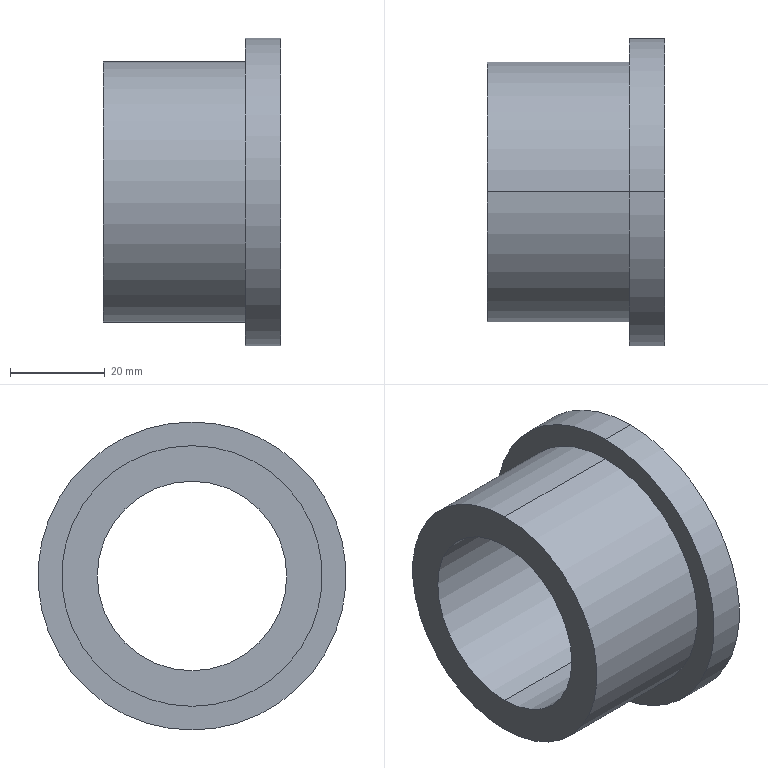Part | SolidWorks | features Revolution 1 | 1 solid | 9 faces | box 37.5 x 65 x 65 mm | volume 49038 mm3 | cylinder 6 | plane 3 | commonest cylinder face diameters 40 x2 55 x2 65 x2
STEP:
#1=CARTESIAN_POINT('',(-7.5,0.,27.5));
#2=VERTEX_POINT('',#1);
#3=CARTESIAN_POINT('',(-7.5,0.,-27.5));
#4=VERTEX_POINT('',#3);
#5=CARTESIAN_POINT('',(-7.5,0.,0.));
#6=DIRECTION('',(-1.,0.,0.));
#7=DIRECTION('',(0.,0.,1.));
#8=AXIS2_PLACEMENT_3D('',#5,#6,#7);
#9=CIRCLE('',#8,27.5);
#10=EDGE_CURVE('',#2,#4,#9,.T.);
#11=ORIENTED_EDGE('',*,*,#10,.T.);
#12=CARTESIAN_POINT('',(-37.5,0.,-27.5));
#13=VERTEX_POINT('',#12);
#14=CARTESIAN_POINT('',(-54.785,0.,-27.5));
#15=DIRECTION('',(-1.,0.,0.));
#16=VECTOR('',#15,1000.);
#17=LINE('',#14,#16);
#18=EDGE_CURVE('',#4,#13,#17,.T.);
#19=ORIENTED_EDGE('',*,*,#18,.T.);
#20=CARTESIAN_POINT('',(-37.5,0.,27.5));
#21=VERTEX_POINT('',#20);
#22=CARTESIAN_POINT('',(-37.5,0.,0.));
#23=DIRECTION('',(-1.,0.,0.));
#24=DIRECTION('',(0.,0.,1.));
#25=AXIS2_PLACEMENT_3D('',#22,#23,#24);
#26=CIRCLE('',#25,27.5);
#27=EDGE_CURVE('',#21,#13,#26,.T.);
#28=ORIENTED_EDGE('',*,*,#27,.F.);
#29=CARTESIAN_POINT('',(-54.785,0.,27.5));
#30=DIRECTION('',(-1.,0.,0.));
#31=VECTOR('',#30,1000.);
#32=LINE('',#29,#31);
#33=EDGE_CURVE('',#2,#21,#32,.T.);
#34=ORIENTED_EDGE('',*,*,#33,.F.);
#35=EDGE_LOOP('',(#11,#19,#28,#34));
#36=FACE_OUTER_BOUND('',#35,.T.);
#37=CARTESIAN_POINT('',(-54.785,0.,0.));
#38=DIRECTION('',(-1.,0.,0.));
#39=DIRECTION('',(0.,0.,1.));
#40=AXIS2_PLACEMENT_3D('',#37,#38,#39);
#41=CYLINDRICAL_SURFACE('',#40,27.5);
#42=ADVANCED_FACE('',(#36),#41,.T.);
#43=CARTESIAN_POINT('',(0.,0.,-20.));
#44=VERTEX_POINT('',#43);
#45=CARTESIAN_POINT('',(0.,0.,20.));
#46=VERTEX_POINT('',#45);
#47=CARTESIAN_POINT('',(0.,0.,0.));
#48=DIRECTION('',(-1.,0.,0.));
#49=DIRECTION('',(0.,0.,1.));
#50=AXIS2_PLACEMENT_3D('',#47,#48,#49);
#51=CIRCLE('',#50,20.);
#52=EDGE_CURVE('',#44,#46,#51,.T.);
#53=ORIENTED_EDGE('',*,*,#52,.F.);
#54=CARTESIAN_POINT('',(-37.5,0.,-20.));
#55=VERTEX_POINT('',#54);
#56=CARTESIAN_POINT('',(-54.785,0.,-20.));
#57=DIRECTION('',(-1.,0.,0.));
#58=VECTOR('',#57,1000.);
#59=LINE('',#56,#58);
#60=EDGE_CURVE('',#44,#55,#59,.T.);
#61=ORIENTED_EDGE('',*,*,#60,.T.);
#62=CARTESIAN_POINT('',(-37.5,0.,20.));
#63=VERTEX_POINT('',#62);
#64=CARTESIAN_POINT('',(-37.5,0.,0.));
#65=DIRECTION('',(-1.,0.,0.));
#66=DIRECTION('',(0.,0.,1.));
#67=AXIS2_PLACEMENT_3D('',#64,#65,#66);
#68=CIRCLE('',#67,20.);
#69=EDGE_CURVE('',#55,#63,#68,.T.);
#70=ORIENTED_EDGE('',*,*,#69,.T.);
#71=CARTESIAN_POINT('',(-54.785,0.,20.));
#72=DIRECTION('',(-1.,0.,0.));
#73=VECTOR('',#72,1000.);
#74=LINE('',#71,#73);
#75=EDGE_CURVE('',#46,#63,#74,.T.);
#76=ORIENTED_EDGE('',*,*,#75,.F.);
#77=EDGE_LOOP('',(#53,#61,#70,#76));
#78=FACE_OUTER_BOUND('',#77,.T.);
#79=CARTESIAN_POINT('',(-54.785,0.,0.));
#80=DIRECTION('',(-1.,0.,0.));
#81=DIRECTION('',(0.,0.,1.));
#82=AXIS2_PLACEMENT_3D('',#79,#80,#81);
#83=CYLINDRICAL_SURFACE('',#82,20.);
#84=ADVANCED_FACE('',(#78),#83,.F.);
#85=CARTESIAN_POINT('',(0.,0.,32.5));
#86=VERTEX_POINT('',#85);
#87=CARTESIAN_POINT('',(0.,0.,-32.5));
#88=VERTEX_POINT('',#87);
#89=CARTESIAN_POINT('',(0.,0.,0.));
#90=DIRECTION('',(-1.,0.,0.));
#91=DIRECTION('',(0.,0.,1.));
#92=AXIS2_PLACEMENT_3D('',#89,#90,#91);
#93=CIRCLE('',#92,32.5);
#94=EDGE_CURVE('',#86,#88,#93,.T.);
#95=ORIENTED_EDGE('',*,*,#94,.T.);
#96=CARTESIAN_POINT('',(-7.5,0.,-32.5));
#97=VERTEX_POINT('',#96);
#98=CARTESIAN_POINT('',(-54.785,0.,-32.5));
#99=DIRECTION('',(-1.,0.,0.));
#100=VECTOR('',#99,1000.);
#101=LINE('',#98,#100);
#102=EDGE_CURVE('',#88,#97,#101,.T.);
#103=ORIENTED_EDGE('',*,*,#102,.T.);
#104=CARTESIAN_POINT('',(-7.5,0.,32.5));
#105=VERTEX_POINT('',#104);
#106=CARTESIAN_POINT('',(-7.5,0.,0.));
#107=DIRECTION('',(-1.,0.,0.));
#108=DIRECTION('',(0.,0.,1.));
#109=AXIS2_PLACEMENT_3D('',#106,#107,#108);
#110=CIRCLE('',#109,32.5);
#111=EDGE_CURVE('',#105,#97,#110,.T.);
#112=ORIENTED_EDGE('',*,*,#111,.F.);
#113=CARTESIAN_POINT('',(-54.785,0.,32.5));
#114=DIRECTION('',(-1.,0.,0.));
#115=VECTOR('',#114,1000.);
#116=LINE('',#113,#115);
#117=EDGE_CURVE('',#86,#105,#116,.T.);
#118=ORIENTED_EDGE('',*,*,#117,.F.);
#119=EDGE_LOOP('',(#95,#103,#112,#118));
#120=FACE_OUTER_BOUND('',#119,.T.);
#121=CARTESIAN_POINT('',(-54.785,0.,0.));
#122=DIRECTION('',(-1.,0.,0.));
#123=DIRECTION('',(0.,0.,1.));
#124=AXIS2_PLACEMENT_3D('',#121,#122,#123);
#125=CYLINDRICAL_SURFACE('',#124,32.5);
#126=ADVANCED_FACE('',(#120),#125,.T.);
#127=ORIENTED_EDGE('',*,*,#102,.F.);
#128=CARTESIAN_POINT('',(0.,0.,0.));
#129=DIRECTION('',(-1.,0.,0.));
#130=DIRECTION('',(0.,0.,1.));
#131=AXIS2_PLACEMENT_3D('',#128,#129,#130);
#132=CIRCLE('',#131,32.5);
#133=EDGE_CURVE('',#88,#86,#132,.T.);
#134=ORIENTED_EDGE('',*,*,#133,.T.);
#135=ORIENTED_EDGE('',*,*,#117,.T.);
#136=CARTESIAN_POINT('',(-7.5,0.,0.));
#137=DIRECTION('',(-1.,0.,0.));
#138=DIRECTION('',(0.,0.,1.));
#139=AXIS2_PLACEMENT_3D('',#136,#137,#138);
#140=CIRCLE('',#139,32.5);
#141=EDGE_CURVE('',#97,#105,#140,.T.);
#142=ORIENTED_EDGE('',*,*,#141,.F.);
#143=EDGE_LOOP('',(#127,#134,#135,#142));
#144=FACE_OUTER_BOUND('',#143,.T.);
#145=CARTESIAN_POINT('',(-54.785,0.,0.));
#146=DIRECTION('',(-1.,0.,0.));
#147=DIRECTION('',(0.,0.,1.));
#148=AXIS2_PLACEMENT_3D('',#145,#146,#147);
#149=CYLINDRICAL_SURFACE('',#148,32.5);
#150=ADVANCED_FACE('',(#144),#149,.T.);
#151=ORIENTED_EDGE('',*,*,#94,.F.);
#152=ORIENTED_EDGE('',*,*,#133,.F.);
#153=EDGE_LOOP('',(#151,#152));
#154=FACE_OUTER_BOUND('',#153,.T.);
#155=CARTESIAN_POINT('',(0.,0.,0.));
#156=DIRECTION('',(-1.,0.,0.));
#157=DIRECTION('',(0.,0.,1.));
#158=AXIS2_PLACEMENT_3D('',#155,#156,#157);
#159=CIRCLE('',#158,20.);
#160=EDGE_CURVE('',#46,#44,#159,.T.);
#161=ORIENTED_EDGE('',*,*,#160,.T.);
#162=ORIENTED_EDGE('',*,*,#52,.T.);
#163=EDGE_LOOP('',(#161,#162));
#164=FACE_BOUND('',#163,.T.);
#165=CARTESIAN_POINT('',(0.,32.5,0.));
#166=DIRECTION('',(-1.,0.,0.));
#167=DIRECTION('',(0.,0.,1.));
#168=AXIS2_PLACEMENT_3D('',#165,#166,#167);
#169=PLANE('',#168);
#170=ADVANCED_FACE('',(#154,#164),#169,.F.);
#171=ORIENTED_EDGE('',*,*,#60,.F.);
#172=ORIENTED_EDGE('',*,*,#160,.F.);
#173=ORIENTED_EDGE('',*,*,#75,.T.);
#174=CARTESIAN_POINT('',(-37.5,0.,0.));
#175=DIRECTION('',(-1.,0.,0.));
#176=DIRECTION('',(0.,0.,1.));
#177=AXIS2_PLACEMENT_3D('',#174,#175,#176);
#178=CIRCLE('',#177,20.);
#179=EDGE_CURVE('',#63,#55,#178,.T.);
#180=ORIENTED_EDGE('',*,*,#179,.T.);
#181=EDGE_LOOP('',(#171,#172,#173,#180));
#182=FACE_OUTER_BOUND('',#181,.T.);
#183=CARTESIAN_POINT('',(-54.785,0.,0.));
#184=DIRECTION('',(-1.,0.,0.));
#185=DIRECTION('',(0.,0.,1.));
#186=AXIS2_PLACEMENT_3D('',#183,#184,#185);
#187=CYLINDRICAL_SURFACE('',#186,20.);
#188=ADVANCED_FACE('',(#182),#187,.F.);
#189=ORIENTED_EDGE('',*,*,#179,.F.);
#190=ORIENTED_EDGE('',*,*,#69,.F.);
#191=EDGE_LOOP('',(#189,#190));
#192=FACE_BOUND('',#191,.T.);
#193=ORIENTED_EDGE('',*,*,#27,.T.);
#194=CARTESIAN_POINT('',(-37.5,0.,0.));
#195=DIRECTION('',(-1.,0.,0.));
#196=DIRECTION('',(0.,0.,1.));
#197=AXIS2_PLACEMENT_3D('',#194,#195,#196);
#198=CIRCLE('',#197,27.5);
#199=EDGE_CURVE('',#13,#21,#198,.T.);
#200=ORIENTED_EDGE('',*,*,#199,.T.);
#201=EDGE_LOOP('',(#193,#200));
#202=FACE_OUTER_BOUND('',#201,.T.);
#203=CARTESIAN_POINT('',(-37.5,20.,0.));
#204=DIRECTION('',(1.,0.,0.));
#205=DIRECTION('',(0.,0.,-1.));
#206=AXIS2_PLACEMENT_3D('',#203,#204,#205);
#207=PLANE('',#206);
#208=ADVANCED_FACE('',(#192,#202),#207,.F.);
#209=ORIENTED_EDGE('',*,*,#18,.F.);
#210=CARTESIAN_POINT('',(-7.5,0.,0.));
#211=DIRECTION('',(-1.,0.,0.));
#212=DIRECTION('',(0.,0.,1.));
#213=AXIS2_PLACEMENT_3D('',#210,#211,#212);
#214=CIRCLE('',#213,27.5);
#215=EDGE_CURVE('',#4,#2,#214,.T.);
#216=ORIENTED_EDGE('',*,*,#215,.T.);
#217=ORIENTED_EDGE('',*,*,#33,.T.);
#218=ORIENTED_EDGE('',*,*,#199,.F.);
#219=EDGE_LOOP('',(#209,#216,#217,#218));
#220=FACE_OUTER_BOUND('',#219,.T.);
#221=CARTESIAN_POINT('',(-54.785,0.,0.));
#222=DIRECTION('',(-1.,0.,0.));
#223=DIRECTION('',(0.,0.,1.));
#224=AXIS2_PLACEMENT_3D('',#221,#222,#223);
#225=CYLINDRICAL_SURFACE('',#224,27.5);
#226=ADVANCED_FACE('',(#220),#225,.T.);
#227=ORIENTED_EDGE('',*,*,#10,.F.);
#228=ORIENTED_EDGE('',*,*,#215,.F.);
#229=EDGE_LOOP('',(#227,#228));
#230=FACE_BOUND('',#229,.T.);
#231=ORIENTED_EDGE('',*,*,#111,.T.);
#232=ORIENTED_EDGE('',*,*,#141,.T.);
#233=EDGE_LOOP('',(#231,#232));
#234=FACE_OUTER_BOUND('',#233,.T.);
#235=CARTESIAN_POINT('',(-7.5,27.5,0.));
#236=DIRECTION('',(1.,0.,0.));
#237=DIRECTION('',(0.,0.,-1.));
#238=AXIS2_PLACEMENT_3D('',#235,#236,#237);
#239=PLANE('',#238);
#240=ADVANCED_FACE('',(#230,#234),#239,.F.);
#241=CLOSED_SHELL('',(#42,#84,#126,#150,#170,#188,#208,#226,#240));
#242=MANIFOLD_SOLID_BREP('',#241);
#243=CARTESIAN_POINT('',(0.,0.,0.));
#244=DIRECTION('',(0.,0.,1.));
#245=DIRECTION('',(1.,0.,0.));
#246=AXIS2_PLACEMENT_3D('',#243,#244,#245);
#247=(LENGTH_UNIT()NAMED_UNIT(*)SI_UNIT(.MILLI.,.METRE.));
#248=UNCERTAINTY_MEASURE_WITH_UNIT(LENGTH_MEASURE(0.00001),#247,'','');
#249=(NAMED_UNIT(*)PLANE_ANGLE_UNIT()SI_UNIT($,.RADIAN.));
#250=(NAMED_UNIT(*)SI_UNIT($,.STERADIAN.)SOLID_ANGLE_UNIT());
#251=(GEOMETRIC_REPRESENTATION_CONTEXT(3)GLOBAL_UNCERTAINTY_ASSIGNED_CONTEXT((#248))GLOBAL_UNIT_ASSIGNED_CONTEXT((#247,#249,#250))REPRESENTATION_CONTEXT('',''));
#252=ADVANCED_BREP_SHAPE_REPRESENTATION('',(#242,#246),#251);